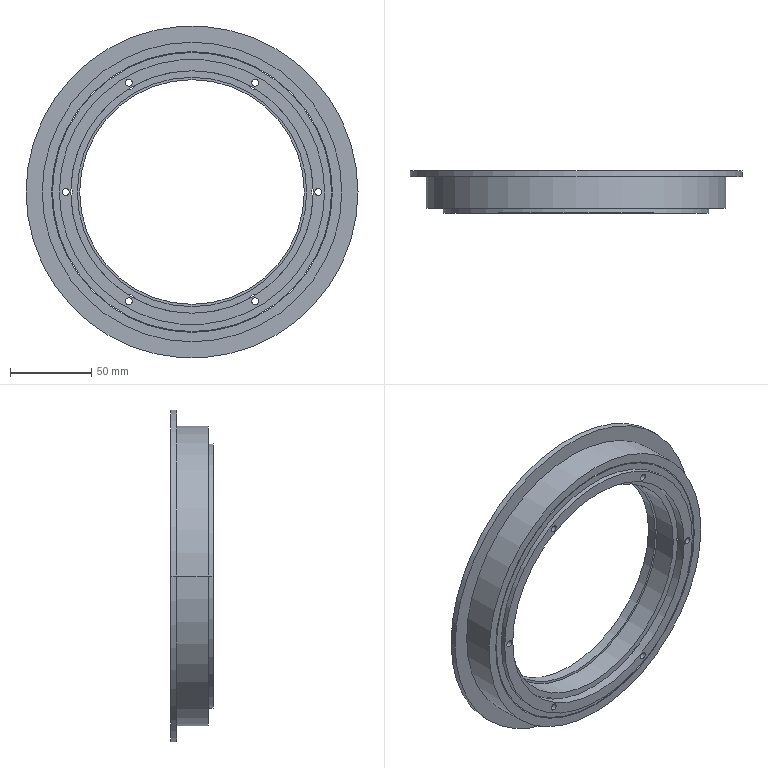Part | SolidWorks | features ICE 2, Revolution 1 | 2 solids | 54 faces | box 204 x 26 x 204 mm | volume 266673 mm3 | cylinder 40 | plane 14 | commonest cylinder face diameters 4.2 x12 8.2 x12 137.991 x2 140.991 x2 148.991 x2 162.991 x2